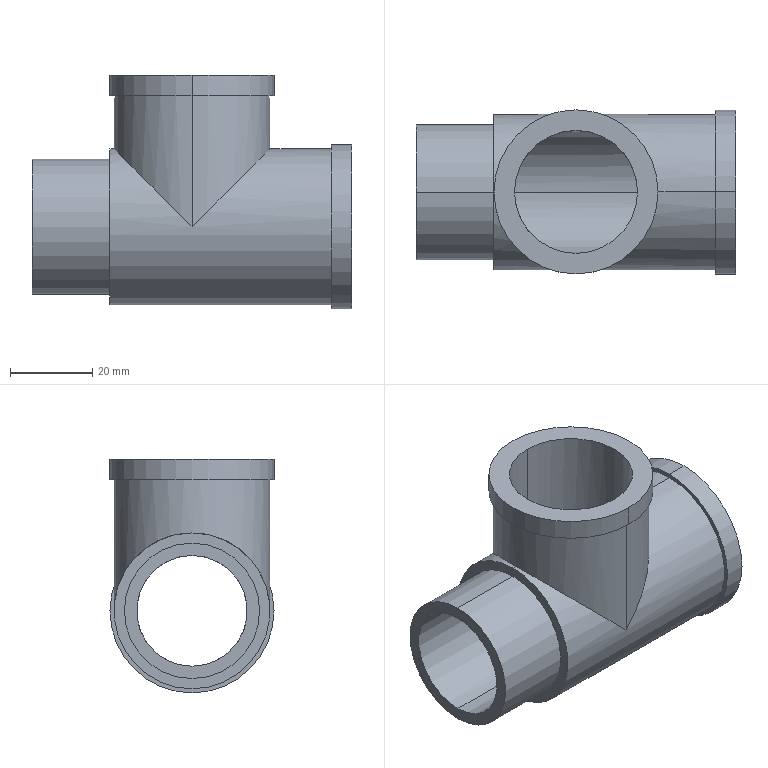Part | SolidWorks | features ICE 2, Revolution 2, Chamfer 1 | 1 solid | 26 faces | box 78 x 40 x 57 mm | volume 38567 mm3 | cylinder 18 | plane 8 | commonest cylinder face diameters 38 x6 30 x4 40 x4 27 x2 33 x2
STEP:
#1=CARTESIAN_POINT('',(78.,0.,-15.));
#2=VERTEX_POINT('',#1);
#3=CARTESIAN_POINT('',(78.,0.,15.));
#4=VERTEX_POINT('',#3);
#5=CARTESIAN_POINT('',(78.,0.,0.));
#6=DIRECTION('',(-1.,0.,0.));
#7=DIRECTION('',(0.,0.,1.));
#8=AXIS2_PLACEMENT_3D('',#5,#6,#7);
#9=CIRCLE('',#8,15.);
#10=EDGE_CURVE('',#2,#4,#9,.T.);
#11=ORIENTED_EDGE('',*,*,#10,.F.);
#12=CARTESIAN_POINT('',(20.,0.,-15.));
#13=VERTEX_POINT('',#12);
#14=CARTESIAN_POINT('',(0.,0.,-15.));
#15=DIRECTION('',(-1.,0.,0.));
#16=VECTOR('',#15,1000.);
#17=LINE('',#14,#16);
#18=EDGE_CURVE('',#2,#13,#17,.T.);
#19=ORIENTED_EDGE('',*,*,#18,.T.);
#20=CARTESIAN_POINT('',(21.,-6.083,-13.711));
#21=VERTEX_POINT('',#20);
#22=CARTESIAN_POINT('',(21.,-6.083,-13.711));
#23=CARTESIAN_POINT('',(20.843,-5.618,-13.918));
#24=CARTESIAN_POINT('',(20.701,-5.138,-14.102));
#25=CARTESIAN_POINT('',(20.455,-4.163,-14.42));
#26=CARTESIAN_POINT('',(20.35,-3.665,-14.555));
#27=CARTESIAN_POINT('',(20.178,-2.646,-14.774));
#28=CARTESIAN_POINT('',(20.112,-2.123,-14.858));
#29=CARTESIAN_POINT('',(20.023,-1.066,-14.972));
#30=CARTESIAN_POINT('',(20.,-0.5331,-15.));
#31=CARTESIAN_POINT('',(20.,0.,-15.));
#32=B_SPLINE_CURVE_WITH_KNOTS('',3,(#22,#23,#24,#25,#26,#27,#28,#29,#30,#31),.UNSPECIFIED.,.F.,.F.,(4,2,2,2,4),(0.09269,0.09426,0.09584,0.09741,0.09898),.UNSPECIFIED.);
#33=EDGE_CURVE('',#21,#13,#32,.T.);
#34=ORIENTED_EDGE('',*,*,#33,.F.);
#35=CARTESIAN_POINT('',(21.,-6.083,13.711));
#36=VERTEX_POINT('',#35);
#37=CARTESIAN_POINT('',(21.,0.,0.));
#38=DIRECTION('',(-1.,0.,0.));
#39=DIRECTION('',(0.,0.,1.));
#40=AXIS2_PLACEMENT_3D('',#37,#38,#39);
#41=CIRCLE('',#40,15.);
#42=EDGE_CURVE('',#21,#36,#41,.T.);
#43=ORIENTED_EDGE('',*,*,#42,.T.);
#44=CARTESIAN_POINT('',(20.,0.,15.));
#45=VERTEX_POINT('',#44);
#46=CARTESIAN_POINT('',(20.,0.,15.));
#47=CARTESIAN_POINT('',(20.,-0.5267,15.));
#48=CARTESIAN_POINT('',(20.022,-1.054,14.972));
#49=CARTESIAN_POINT('',(20.088,-1.844,14.889));
#50=CARTESIAN_POINT('',(20.116,-2.109,14.853));
#51=CARTESIAN_POINT('',(20.181,-2.632,14.77));
#52=CARTESIAN_POINT('',(20.219,-2.89,14.721));
#53=CARTESIAN_POINT('',(20.348,-3.657,14.557));
#54=CARTESIAN_POINT('',(20.453,-4.157,14.422));
#55=CARTESIAN_POINT('',(20.7,-5.136,14.103));
#56=CARTESIAN_POINT('',(20.843,-5.617,13.918));
#57=CARTESIAN_POINT('',(21.,-6.083,13.711));
#58=B_SPLINE_CURVE_WITH_KNOTS('',3,(#46,#47,#48,#49,#50,#51,#52,#53,#54,#55,#56,#57),.UNSPECIFIED.,.F.,.F.,(4,2,2,2,2,4),(0.04955,0.05113,0.05192,0.05271,0.05429,0.05587),.UNSPECIFIED.);
#59=EDGE_CURVE('',#45,#36,#58,.T.);
#60=ORIENTED_EDGE('',*,*,#59,.F.);
#61=CARTESIAN_POINT('',(24.,0.,15.));
#62=VERTEX_POINT('',#61);
#63=CARTESIAN_POINT('',(0.,0.,15.));
#64=DIRECTION('',(-1.,0.,0.));
#65=VECTOR('',#64,1000.);
#66=LINE('',#63,#65);
#67=EDGE_CURVE('',#62,#45,#66,.T.);
#68=ORIENTED_EDGE('',*,*,#67,.F.);
#69=CARTESIAN_POINT('',(39.,-15.,0.));
#70=VERTEX_POINT('',#69);
#71=CARTESIAN_POINT('',(39.,-15.,0.));
#72=CARTESIAN_POINT('',(30.213,-15.,8.787));
#73=CARTESIAN_POINT('',(24.,-8.787,15.));
#74=CARTESIAN_POINT('',(24.,0.,15.));
#75=(BOUNDED_CURVE()B_SPLINE_CURVE(3,(#71,#72,#73,#74),.UNSPECIFIED.,.F.,.F.)B_SPLINE_CURVE_WITH_KNOTS((4,4),(4.712,6.283),.UNSPECIFIED.)CURVE()GEOMETRIC_REPRESENTATION_ITEM()RATIONAL_B_SPLINE_CURVE((1.,0.8047,0.8047,1.))REPRESENTATION_ITEM(''));
#76=EDGE_CURVE('',#70,#62,#75,.T.);
#77=ORIENTED_EDGE('',*,*,#76,.F.);
#78=CARTESIAN_POINT('',(54.,0.,15.));
#79=VERTEX_POINT('',#78);
#80=CARTESIAN_POINT('',(54.,0.,15.));
#81=CARTESIAN_POINT('',(54.,-8.787,15.));
#82=CARTESIAN_POINT('',(47.787,-15.,8.787));
#83=CARTESIAN_POINT('',(39.,-15.,0.));
#84=(BOUNDED_CURVE()B_SPLINE_CURVE(3,(#80,#81,#82,#83),.UNSPECIFIED.,.F.,.F.)B_SPLINE_CURVE_WITH_KNOTS((4,4),(0.,1.571),.UNSPECIFIED.)CURVE()GEOMETRIC_REPRESENTATION_ITEM()RATIONAL_B_SPLINE_CURVE((1.,0.8047,0.8047,1.))REPRESENTATION_ITEM(''));
#85=EDGE_CURVE('',#79,#70,#84,.T.);
#86=ORIENTED_EDGE('',*,*,#85,.F.);
#87=CARTESIAN_POINT('',(0.,0.,15.));
#88=DIRECTION('',(-1.,0.,0.));
#89=VECTOR('',#88,1000.);
#90=LINE('',#87,#89);
#91=EDGE_CURVE('',#4,#79,#90,.T.);
#92=ORIENTED_EDGE('',*,*,#91,.F.);
#93=EDGE_LOOP('',(#11,#19,#34,#43,#60,#68,#77,#86,#92));
#94=FACE_OUTER_BOUND('',#93,.T.);
#95=CARTESIAN_POINT('',(0.,0.,0.));
#96=DIRECTION('',(-1.,0.,0.));
#97=DIRECTION('',(0.,0.,1.));
#98=AXIS2_PLACEMENT_3D('',#95,#96,#97);
#99=CYLINDRICAL_SURFACE('',#98,15.);
#100=ADVANCED_FACE('',(#94),#99,.F.);
#101=CARTESIAN_POINT('',(39.,-15.,37.));
#102=VERTEX_POINT('',#101);
#103=CARTESIAN_POINT('',(39.,15.,37.));
#104=VERTEX_POINT('',#103);
#105=CARTESIAN_POINT('',(39.,0.,37.));
#106=DIRECTION('',(0.,0.,-1.));
#107=DIRECTION('',(0.,1.,0.));
#108=AXIS2_PLACEMENT_3D('',#105,#106,#107);
#109=CIRCLE('',#108,15.);
#110=EDGE_CURVE('',#102,#104,#109,.T.);
#111=ORIENTED_EDGE('',*,*,#110,.F.);
#112=CARTESIAN_POINT('',(39.,-15.,0.));
#113=DIRECTION('',(0.,0.,-1.));
#114=VECTOR('',#113,1000.);
#115=LINE('',#112,#114);
#116=EDGE_CURVE('',#102,#70,#115,.T.);
#117=ORIENTED_EDGE('',*,*,#116,.T.);
#118=ORIENTED_EDGE('',*,*,#76,.T.);
#119=CARTESIAN_POINT('',(39.,15.,0.));
#120=VERTEX_POINT('',#119);
#121=CARTESIAN_POINT('',(24.,0.,15.));
#122=CARTESIAN_POINT('',(24.,8.787,15.));
#123=CARTESIAN_POINT('',(30.213,15.,8.787));
#124=CARTESIAN_POINT('',(39.,15.,0.));
#125=(BOUNDED_CURVE()B_SPLINE_CURVE(3,(#121,#122,#123,#124),.UNSPECIFIED.,.F.,.F.)B_SPLINE_CURVE_WITH_KNOTS((4,4),(0.,1.571),.UNSPECIFIED.)CURVE()GEOMETRIC_REPRESENTATION_ITEM()RATIONAL_B_SPLINE_CURVE((1.,0.8047,0.8047,1.))REPRESENTATION_ITEM(''));
#126=EDGE_CURVE('',#62,#120,#125,.T.);
#127=ORIENTED_EDGE('',*,*,#126,.T.);
#128=CARTESIAN_POINT('',(39.,15.,0.));
#129=DIRECTION('',(0.,0.,-1.));
#130=VECTOR('',#129,1000.);
#131=LINE('',#128,#130);
#132=EDGE_CURVE('',#104,#120,#131,.T.);
#133=ORIENTED_EDGE('',*,*,#132,.F.);
#134=EDGE_LOOP('',(#111,#117,#118,#127,#133));
#135=FACE_OUTER_BOUND('',#134,.T.);
#136=CARTESIAN_POINT('',(39.,0.,0.));
#137=DIRECTION('',(0.,0.,-1.));
#138=DIRECTION('',(0.,1.,0.));
#139=AXIS2_PLACEMENT_3D('',#136,#137,#138);
#140=CYLINDRICAL_SURFACE('',#139,15.);
#141=ADVANCED_FACE('',(#135),#140,.F.);
#142=CARTESIAN_POINT('',(39.,19.,32.));
#143=VERTEX_POINT('',#142);
#144=CARTESIAN_POINT('',(39.,-19.,32.));
#145=VERTEX_POINT('',#144);
#146=CARTESIAN_POINT('',(39.,0.,32.));
#147=DIRECTION('',(0.,0.,-1.));
#148=DIRECTION('',(0.,1.,0.));
#149=AXIS2_PLACEMENT_3D('',#146,#147,#148);
#150=CIRCLE('',#149,19.);
#151=EDGE_CURVE('',#143,#145,#150,.T.);
#152=ORIENTED_EDGE('',*,*,#151,.T.);
#153=CARTESIAN_POINT('',(39.,-19.,0.));
#154=VERTEX_POINT('',#153);
#155=CARTESIAN_POINT('',(39.,-19.,0.));
#156=DIRECTION('',(0.,0.,-1.));
#157=VECTOR('',#156,1000.);
#158=LINE('',#155,#157);
#159=EDGE_CURVE('',#145,#154,#158,.T.);
#160=ORIENTED_EDGE('',*,*,#159,.T.);
#161=CARTESIAN_POINT('',(58.,0.,19.));
#162=VERTEX_POINT('',#161);
#163=CARTESIAN_POINT('',(39.,-19.,0.));
#164=CARTESIAN_POINT('',(50.13,-19.,11.13));
#165=CARTESIAN_POINT('',(58.,-11.13,19.));
#166=CARTESIAN_POINT('',(58.,0.,19.));
#167=(BOUNDED_CURVE()B_SPLINE_CURVE(3,(#163,#164,#165,#166),.UNSPECIFIED.,.F.,.T.)B_SPLINE_CURVE_WITH_KNOTS((4,4),(1.571,3.142),.UNSPECIFIED.)CURVE()GEOMETRIC_REPRESENTATION_ITEM()RATIONAL_B_SPLINE_CURVE((1.,0.8047,0.8047,1.))REPRESENTATION_ITEM(''));
#168=EDGE_CURVE('',#154,#162,#167,.T.);
#169=ORIENTED_EDGE('',*,*,#168,.T.);
#170=CARTESIAN_POINT('',(39.,19.,0.));
#171=VERTEX_POINT('',#170);
#172=CARTESIAN_POINT('',(58.,0.,19.));
#173=CARTESIAN_POINT('',(58.,11.13,19.));
#174=CARTESIAN_POINT('',(50.13,19.,11.13));
#175=CARTESIAN_POINT('',(39.,19.,0.));
#176=(BOUNDED_CURVE()B_SPLINE_CURVE(3,(#172,#173,#174,#175),.UNSPECIFIED.,.F.,.F.)B_SPLINE_CURVE_WITH_KNOTS((4,4),(3.142,4.712),.UNSPECIFIED.)CURVE()GEOMETRIC_REPRESENTATION_ITEM()RATIONAL_B_SPLINE_CURVE((1.,0.8047,0.8047,1.))REPRESENTATION_ITEM(''));
#177=EDGE_CURVE('',#162,#171,#176,.T.);
#178=ORIENTED_EDGE('',*,*,#177,.T.);
#179=CARTESIAN_POINT('',(39.,19.,0.));
#180=DIRECTION('',(0.,0.,-1.));
#181=VECTOR('',#180,1000.);
#182=LINE('',#179,#181);
#183=EDGE_CURVE('',#143,#171,#182,.T.);
#184=ORIENTED_EDGE('',*,*,#183,.F.);
#185=EDGE_LOOP('',(#152,#160,#169,#178,#184));
#186=FACE_OUTER_BOUND('',#185,.T.);
#187=CARTESIAN_POINT('',(39.,0.,0.));
#188=DIRECTION('',(0.,0.,-1.));
#189=DIRECTION('',(0.,1.,0.));
#190=AXIS2_PLACEMENT_3D('',#187,#188,#189);
#191=CYLINDRICAL_SURFACE('',#190,19.);
#192=ADVANCED_FACE('',(#186),#191,.T.);
#193=CARTESIAN_POINT('',(39.,20.,37.));
#194=VERTEX_POINT('',#193);
#195=CARTESIAN_POINT('',(39.,-20.,37.));
#196=VERTEX_POINT('',#195);
#197=CARTESIAN_POINT('',(39.,0.,37.));
#198=DIRECTION('',(0.,0.,-1.));
#199=DIRECTION('',(0.,1.,0.));
#200=AXIS2_PLACEMENT_3D('',#197,#198,#199);
#201=CIRCLE('',#200,20.);
#202=EDGE_CURVE('',#194,#196,#201,.T.);
#203=ORIENTED_EDGE('',*,*,#202,.T.);
#204=CARTESIAN_POINT('',(39.,-20.,32.));
#205=VERTEX_POINT('',#204);
#206=CARTESIAN_POINT('',(39.,-20.,0.));
#207=DIRECTION('',(0.,0.,-1.));
#208=VECTOR('',#207,1000.);
#209=LINE('',#206,#208);
#210=EDGE_CURVE('',#196,#205,#209,.T.);
#211=ORIENTED_EDGE('',*,*,#210,.T.);
#212=CARTESIAN_POINT('',(39.,20.,32.));
#213=VERTEX_POINT('',#212);
#214=CARTESIAN_POINT('',(39.,0.,32.));
#215=DIRECTION('',(0.,0.,-1.));
#216=DIRECTION('',(0.,1.,0.));
#217=AXIS2_PLACEMENT_3D('',#214,#215,#216);
#218=CIRCLE('',#217,20.);
#219=EDGE_CURVE('',#213,#205,#218,.T.);
#220=ORIENTED_EDGE('',*,*,#219,.F.);
#221=CARTESIAN_POINT('',(39.,20.,0.));
#222=DIRECTION('',(0.,0.,-1.));
#223=VECTOR('',#222,1000.);
#224=LINE('',#221,#223);
#225=EDGE_CURVE('',#194,#213,#224,.T.);
#226=ORIENTED_EDGE('',*,*,#225,.F.);
#227=EDGE_LOOP('',(#203,#211,#220,#226));
#228=FACE_OUTER_BOUND('',#227,.T.);
#229=CARTESIAN_POINT('',(39.,0.,0.));
#230=DIRECTION('',(0.,0.,-1.));
#231=DIRECTION('',(0.,1.,0.));
#232=AXIS2_PLACEMENT_3D('',#229,#230,#231);
#233=CYLINDRICAL_SURFACE('',#232,20.);
#234=ADVANCED_FACE('',(#228),#233,.T.);
#235=CARTESIAN_POINT('',(78.,0.,20.));
#236=VERTEX_POINT('',#235);
#237=CARTESIAN_POINT('',(78.,0.,-20.));
#238=VERTEX_POINT('',#237);
#239=CARTESIAN_POINT('',(78.,0.,0.));
#240=DIRECTION('',(-1.,0.,0.));
#241=DIRECTION('',(0.,0.,1.));
#242=AXIS2_PLACEMENT_3D('',#239,#240,#241);
#243=CIRCLE('',#242,20.);
#244=EDGE_CURVE('',#236,#238,#243,.T.);
#245=ORIENTED_EDGE('',*,*,#244,.T.);
#246=CARTESIAN_POINT('',(73.,0.,-20.));
#247=VERTEX_POINT('',#246);
#248=CARTESIAN_POINT('',(0.,0.,-20.));
#249=DIRECTION('',(-1.,0.,0.));
#250=VECTOR('',#249,1000.);
#251=LINE('',#248,#250);
#252=EDGE_CURVE('',#238,#247,#251,.T.);
#253=ORIENTED_EDGE('',*,*,#252,.T.);
#254=CARTESIAN_POINT('',(73.,0.,20.));
#255=VERTEX_POINT('',#254);
#256=CARTESIAN_POINT('',(73.,0.,0.));
#257=DIRECTION('',(-1.,0.,0.));
#258=DIRECTION('',(0.,0.,1.));
#259=AXIS2_PLACEMENT_3D('',#256,#257,#258);
#260=CIRCLE('',#259,20.);
#261=EDGE_CURVE('',#255,#247,#260,.T.);
#262=ORIENTED_EDGE('',*,*,#261,.F.);
#263=CARTESIAN_POINT('',(0.,0.,20.));
#264=DIRECTION('',(-1.,0.,0.));
#265=VECTOR('',#264,1000.);
#266=LINE('',#263,#265);
#267=EDGE_CURVE('',#236,#255,#266,.T.);
#268=ORIENTED_EDGE('',*,*,#267,.F.);
#269=EDGE_LOOP('',(#245,#253,#262,#268));
#270=FACE_OUTER_BOUND('',#269,.T.);
#271=CARTESIAN_POINT('',(0.,0.,0.));
#272=DIRECTION('',(-1.,0.,0.));
#273=DIRECTION('',(0.,0.,1.));
#274=AXIS2_PLACEMENT_3D('',#271,#272,#273);
#275=CYLINDRICAL_SURFACE('',#274,20.);
#276=ADVANCED_FACE('',(#270),#275,.T.);
#277=CARTESIAN_POINT('',(19.,0.,16.5));
#278=VERTEX_POINT('',#277);
#279=CARTESIAN_POINT('',(19.,0.,-16.5));
#280=VERTEX_POINT('',#279);
#281=CARTESIAN_POINT('',(19.,0.,0.));
#282=DIRECTION('',(-1.,0.,0.));
#283=DIRECTION('',(0.,0.,1.));
#284=AXIS2_PLACEMENT_3D('',#281,#282,#283);
#285=CIRCLE('',#284,16.5);
#286=EDGE_CURVE('',#278,#280,#285,.T.);
#287=ORIENTED_EDGE('',*,*,#286,.T.);
#288=CARTESIAN_POINT('',(0.,0.,-16.5));
#289=VERTEX_POINT('',#288);
#290=CARTESIAN_POINT('',(0.,0.,-16.5));
#291=DIRECTION('',(-1.,0.,0.));
#292=VECTOR('',#291,1000.);
#293=LINE('',#290,#292);
#294=EDGE_CURVE('',#280,#289,#293,.T.);
#295=ORIENTED_EDGE('',*,*,#294,.T.);
#296=CARTESIAN_POINT('',(0.,0.,16.5));
#297=VERTEX_POINT('',#296);
#298=CARTESIAN_POINT('',(0.,0.,0.));
#299=DIRECTION('',(-1.,0.,0.));
#300=DIRECTION('',(0.,0.,1.));
#301=AXIS2_PLACEMENT_3D('',#298,#299,#300);
#302=CIRCLE('',#301,16.5);
#303=EDGE_CURVE('',#297,#289,#302,.T.);
#304=ORIENTED_EDGE('',*,*,#303,.F.);
#305=CARTESIAN_POINT('',(0.,0.,16.5));
#306=DIRECTION('',(-1.,0.,0.));
#307=VECTOR('',#306,1000.);
#308=LINE('',#305,#307);
#309=EDGE_CURVE('',#278,#297,#308,.T.);
#310=ORIENTED_EDGE('',*,*,#309,.F.);
#311=EDGE_LOOP('',(#287,#295,#304,#310));
#312=FACE_OUTER_BOUND('',#311,.T.);
#313=CARTESIAN_POINT('',(0.,0.,0.));
#314=DIRECTION('',(-1.,0.,0.));
#315=DIRECTION('',(0.,0.,1.));
#316=AXIS2_PLACEMENT_3D('',#313,#314,#315);
#317=CYLINDRICAL_SURFACE('',#316,16.5);
#318=ADVANCED_FACE('',(#312),#317,.T.);
#319=CARTESIAN_POINT('',(73.,0.,19.));
#320=VERTEX_POINT('',#319);
#321=CARTESIAN_POINT('',(73.,0.,-19.));
#322=VERTEX_POINT('',#321);
#323=CARTESIAN_POINT('',(73.,0.,0.));
#324=DIRECTION('',(-1.,0.,0.));
#325=DIRECTION('',(0.,0.,1.));
#326=AXIS2_PLACEMENT_3D('',#323,#324,#325);
#327=CIRCLE('',#326,19.);
#328=EDGE_CURVE('',#320,#322,#327,.T.);
#329=ORIENTED_EDGE('',*,*,#328,.T.);
#330=CARTESIAN_POINT('',(19.,0.,-19.));
#331=VERTEX_POINT('',#330);
#332=CARTESIAN_POINT('',(0.,0.,-19.));
#333=DIRECTION('',(-1.,0.,0.));
#334=VECTOR('',#333,1000.);
#335=LINE('',#332,#334);
#336=EDGE_CURVE('',#322,#331,#335,.T.);
#337=ORIENTED_EDGE('',*,*,#336,.T.);
#338=CARTESIAN_POINT('',(19.,0.,19.));
#339=VERTEX_POINT('',#338);
#340=CARTESIAN_POINT('',(19.,0.,0.));
#341=DIRECTION('',(-1.,0.,0.));
#342=DIRECTION('',(0.,0.,1.));
#343=AXIS2_PLACEMENT_3D('',#340,#341,#342);
#344=CIRCLE('',#343,19.);
#345=EDGE_CURVE('',#339,#331,#344,.T.);
#346=ORIENTED_EDGE('',*,*,#345,.F.);
#347=CARTESIAN_POINT('',(20.,0.,19.));
#348=VERTEX_POINT('',#347);
#349=CARTESIAN_POINT('',(0.,0.,19.));
#350=DIRECTION('',(-1.,0.,0.));
#351=VECTOR('',#350,1000.);
#352=LINE('',#349,#351);
#353=EDGE_CURVE('',#348,#339,#352,.T.);
#354=ORIENTED_EDGE('',*,*,#353,.F.);
#355=CARTESIAN_POINT('',(39.,19.,0.));
#356=CARTESIAN_POINT('',(27.87,19.,11.13));
#357=CARTESIAN_POINT('',(20.,11.13,19.));
#358=CARTESIAN_POINT('',(20.,0.,19.));
#359=(BOUNDED_CURVE()B_SPLINE_CURVE(3,(#355,#356,#357,#358),.UNSPECIFIED.,.F.,.F.)B_SPLINE_CURVE_WITH_KNOTS((4,4),(4.712,6.283),.UNSPECIFIED.)CURVE()GEOMETRIC_REPRESENTATION_ITEM()RATIONAL_B_SPLINE_CURVE((1.,0.8047,0.8047,1.))REPRESENTATION_ITEM(''));
#360=EDGE_CURVE('',#171,#348,#359,.T.);
#361=ORIENTED_EDGE('',*,*,#360,.F.);
#362=ORIENTED_EDGE('',*,*,#177,.F.);
#363=CARTESIAN_POINT('',(0.,0.,19.));
#364=DIRECTION('',(-1.,0.,0.));
#365=VECTOR('',#364,1000.);
#366=LINE('',#363,#365);
#367=EDGE_CURVE('',#320,#162,#366,.T.);
#368=ORIENTED_EDGE('',*,*,#367,.F.);
#369=EDGE_LOOP('',(#329,#337,#346,#354,#361,#362,#368));
#370=FACE_OUTER_BOUND('',#369,.T.);
#371=CARTESIAN_POINT('',(0.,0.,0.));
#372=DIRECTION('',(-1.,0.,0.));
#373=DIRECTION('',(0.,0.,1.));
#374=AXIS2_PLACEMENT_3D('',#371,#372,#373);
#375=CYLINDRICAL_SURFACE('',#374,19.);
#376=ADVANCED_FACE('',(#370),#375,.T.);
#377=CARTESIAN_POINT('',(20.,0.,-13.5));
#378=VERTEX_POINT('',#377);
#379=CARTESIAN_POINT('',(21.,-6.083,-12.052));
#380=VERTEX_POINT('',#379);
#381=CARTESIAN_POINT('',(20.,0.,-13.5));
#382=CARTESIAN_POINT('',(20.,-0.5304,-13.5));
#383=CARTESIAN_POINT('',(20.022,-1.064,-13.469));
#384=CARTESIAN_POINT('',(20.112,-2.128,-13.342));
#385=CARTESIAN_POINT('',(20.178,-2.649,-13.248));
#386=CARTESIAN_POINT('',(20.35,-3.668,-13.003));
#387=CARTESIAN_POINT('',(20.456,-4.168,-12.851));
#388=CARTESIAN_POINT('',(20.703,-5.146,-12.492));
#389=CARTESIAN_POINT('',(20.845,-5.623,-12.284));
#390=CARTESIAN_POINT('',(21.,-6.083,-12.052));
#391=B_SPLINE_CURVE_WITH_KNOTS('',3,(#381,#382,#383,#384,#385,#386,#387,#388,#389,#390),.UNSPECIFIED.,.F.,.F.,(4,2,2,2,4),(0.006389,0.007982,0.009575,0.01117,0.01276),.UNSPECIFIED.);
#392=EDGE_CURVE('',#378,#380,#391,.T.);
#393=ORIENTED_EDGE('',*,*,#392,.F.);
#394=CARTESIAN_POINT('',(0.,0.,-13.5));
#395=VERTEX_POINT('',#394);
#396=CARTESIAN_POINT('',(0.,0.,-13.5));
#397=DIRECTION('',(-1.,0.,0.));
#398=VECTOR('',#397,1000.);
#399=LINE('',#396,#398);
#400=EDGE_CURVE('',#378,#395,#399,.T.);
#401=ORIENTED_EDGE('',*,*,#400,.T.);
#402=CARTESIAN_POINT('',(0.,0.,13.5));
#403=VERTEX_POINT('',#402);
#404=CARTESIAN_POINT('',(0.,0.,0.));
#405=DIRECTION('',(-1.,0.,0.));
#406=DIRECTION('',(0.,0.,1.));
#407=AXIS2_PLACEMENT_3D('',#404,#405,#406);
#408=CIRCLE('',#407,13.5);
#409=EDGE_CURVE('',#395,#403,#408,.T.);
#410=ORIENTED_EDGE('',*,*,#409,.T.);
#411=CARTESIAN_POINT('',(20.,0.,13.5));
#412=VERTEX_POINT('',#411);
#413=CARTESIAN_POINT('',(0.,0.,13.5));
#414=DIRECTION('',(-1.,0.,0.));
#415=VECTOR('',#414,1000.);
#416=LINE('',#413,#415);
#417=EDGE_CURVE('',#412,#403,#416,.T.);
#418=ORIENTED_EDGE('',*,*,#417,.F.);
#419=CARTESIAN_POINT('',(21.,-6.083,12.052));
#420=VERTEX_POINT('',#419);
#421=CARTESIAN_POINT('',(21.,-6.083,12.052));
#422=CARTESIAN_POINT('',(20.847,-5.631,12.28));
#423=CARTESIAN_POINT('',(20.708,-5.162,12.485));
#424=CARTESIAN_POINT('',(20.46,-4.187,12.845));
#425=CARTESIAN_POINT('',(20.352,-3.677,13.));
#426=CARTESIAN_POINT('',(20.178,-2.649,13.248));
#427=CARTESIAN_POINT('',(20.112,-2.129,13.342));
#428=CARTESIAN_POINT('',(20.023,-1.075,13.468));
#429=CARTESIAN_POINT('',(20.,-0.5395,13.5));
#430=CARTESIAN_POINT('',(20.,0.,13.5));
#431=B_SPLINE_CURVE_WITH_KNOTS('',3,(#421,#422,#423,#424,#425,#426,#427,#428,#429,#430),.UNSPECIFIED.,.F.,.F.,(4,2,2,2,4),(0.08145,0.08304,0.08463,0.08622,0.08782),.UNSPECIFIED.);
#432=EDGE_CURVE('',#420,#412,#431,.T.);
#433=ORIENTED_EDGE('',*,*,#432,.F.);
#434=CARTESIAN_POINT('',(21.,0.,0.));
#435=DIRECTION('',(-1.,0.,0.));
#436=DIRECTION('',(0.,0.,1.));
#437=AXIS2_PLACEMENT_3D('',#434,#435,#436);
#438=CIRCLE('',#437,13.5);
#439=EDGE_CURVE('',#380,#420,#438,.T.);
#440=ORIENTED_EDGE('',*,*,#439,.F.);
#441=EDGE_LOOP('',(#393,#401,#410,#418,#433,#440));
#442=FACE_OUTER_BOUND('',#441,.T.);
#443=CARTESIAN_POINT('',(0.,0.,0.));
#444=DIRECTION('',(-1.,0.,0.));
#445=DIRECTION('',(0.,0.,1.));
#446=AXIS2_PLACEMENT_3D('',#443,#444,#445);
#447=CYLINDRICAL_SURFACE('',#446,13.5);
#448=ADVANCED_FACE('',(#442),#447,.F.);
#449=ORIENTED_EDGE('',*,*,#400,.F.);
#450=CARTESIAN_POINT('',(21.,6.083,-12.052));
#451=VERTEX_POINT('',#450);
#452=CARTESIAN_POINT('',(21.,6.083,-12.052));
#453=CARTESIAN_POINT('',(20.689,5.161,-12.517));
#454=CARTESIAN_POINT('',(20.438,4.19,-12.877));
#455=CARTESIAN_POINT('',(20.178,2.649,-13.248));
#456=CARTESIAN_POINT('',(20.111,2.119,-13.343));
#457=CARTESIAN_POINT('',(20.022,1.062,-13.469));
#458=CARTESIAN_POINT('',(20.,0.5319,-13.5));
#459=CARTESIAN_POINT('',(20.,0.,-13.5));
#460=B_SPLINE_CURVE_WITH_KNOTS('',3,(#452,#453,#454,#455,#456,#457,#458,#459),.UNSPECIFIED.,.F.,.F.,(4,2,2,4),(0.,0.003195,0.004792,0.006389),.UNSPECIFIED.);
#461=EDGE_CURVE('',#451,#378,#460,.T.);
#462=ORIENTED_EDGE('',*,*,#461,.F.);
#463=CARTESIAN_POINT('',(21.,6.083,12.052));
#464=VERTEX_POINT('',#463);
#465=CARTESIAN_POINT('',(21.,0.,0.));
#466=DIRECTION('',(-1.,0.,0.));
#467=DIRECTION('',(0.,0.,1.));
#468=AXIS2_PLACEMENT_3D('',#465,#466,#467);
#469=CIRCLE('',#468,13.5);
#470=EDGE_CURVE('',#464,#451,#469,.T.);
#471=ORIENTED_EDGE('',*,*,#470,.F.);
#472=CARTESIAN_POINT('',(20.,0.,13.5));
#473=CARTESIAN_POINT('',(20.,1.08,13.5));
#474=CARTESIAN_POINT('',(20.091,2.132,13.372));
#475=CARTESIAN_POINT('',(20.351,3.67,13.002));
#476=CARTESIAN_POINT('',(20.458,4.179,12.848));
#477=CARTESIAN_POINT('',(20.706,5.156,12.488));
#478=CARTESIAN_POINT('',(20.846,5.627,12.282));
#479=CARTESIAN_POINT('',(21.,6.083,12.052));
#480=B_SPLINE_CURVE_WITH_KNOTS('',3,(#472,#473,#474,#475,#476,#477,#478,#479),.UNSPECIFIED.,.F.,.F.,(4,2,2,4),(0.,0.003188,0.004782,0.006376),.UNSPECIFIED.);
#481=EDGE_CURVE('',#412,#464,#480,.T.);
#482=ORIENTED_EDGE('',*,*,#481,.F.);
#483=ORIENTED_EDGE('',*,*,#417,.T.);
#484=CARTESIAN_POINT('',(0.,0.,0.));
#485=DIRECTION('',(-1.,0.,0.));
#486=DIRECTION('',(0.,0.,1.));
#487=AXIS2_PLACEMENT_3D('',#484,#485,#486);
#488=CIRCLE('',#487,13.5);
#489=EDGE_CURVE('',#403,#395,#488,.T.);
#490=ORIENTED_EDGE('',*,*,#489,.T.);
#491=EDGE_LOOP('',(#449,#462,#471,#482,#483,#490));
#492=FACE_OUTER_BOUND('',#491,.T.);
#493=CARTESIAN_POINT('',(0.,0.,0.));
#494=DIRECTION('',(-1.,0.,0.));
#495=DIRECTION('',(0.,0.,1.));
#496=AXIS2_PLACEMENT_3D('',#493,#494,#495);
#497=CYLINDRICAL_SURFACE('',#496,13.5);
#498=ADVANCED_FACE('',(#492),#497,.F.);
#499=CARTESIAN_POINT('',(21.,6.083,-13.711));
#500=VERTEX_POINT('',#499);
#501=CARTESIAN_POINT('',(21.,6.083,0.));
#502=DIRECTION('',(0.,0.,1.));
#503=VECTOR('',#502,1000.);
#504=LINE('',#501,#503);
#505=EDGE_CURVE('',#500,#451,#504,.T.);
#506=ORIENTED_EDGE('',*,*,#505,.F.);
#507=CARTESIAN_POINT('',(21.,6.083,13.711));
#508=VERTEX_POINT('',#507);
#509=CARTESIAN_POINT('',(21.,0.,0.));
#510=DIRECTION('',(-1.,0.,0.));
#511=DIRECTION('',(0.,0.,1.));
#512=AXIS2_PLACEMENT_3D('',#509,#510,#511);
#513=CIRCLE('',#512,15.);
#514=EDGE_CURVE('',#508,#500,#513,.T.);
#515=ORIENTED_EDGE('',*,*,#514,.F.);
#516=CARTESIAN_POINT('',(21.,6.083,0.));
#517=DIRECTION('',(0.,0.,1.));
#518=VECTOR('',#517,1000.);
#519=LINE('',#516,#518);
#520=EDGE_CURVE('',#464,#508,#519,.T.);
#521=ORIENTED_EDGE('',*,*,#520,.F.);
#522=ORIENTED_EDGE('',*,*,#470,.T.);
#523=EDGE_LOOP('',(#506,#515,#521,#522));
#524=FACE_OUTER_BOUND('',#523,.T.);
#525=CARTESIAN_POINT('',(21.,15.,0.));
#526=DIRECTION('',(-1.,0.,0.));
#527=DIRECTION('',(0.,0.,1.));
#528=AXIS2_PLACEMENT_3D('',#525,#526,#527);
#529=PLANE('',#528);
#530=ADVANCED_FACE('',(#524),#529,.F.);
#531=CARTESIAN_POINT('',(21.,-6.083,0.));
#532=DIRECTION('',(0.,0.,-1.));
#533=VECTOR('',#532,1000.);
#534=LINE('',#531,#533);
#535=EDGE_CURVE('',#380,#21,#534,.T.);
#536=ORIENTED_EDGE('',*,*,#535,.F.);
#537=ORIENTED_EDGE('',*,*,#439,.T.);
#538=CARTESIAN_POINT('',(21.,-6.083,0.));
#539=DIRECTION('',(0.,0.,-1.));
#540=VECTOR('',#539,1000.);
#541=LINE('',#538,#540);
#542=EDGE_CURVE('',#36,#420,#541,.T.);
#543=ORIENTED_EDGE('',*,*,#542,.F.);
#544=ORIENTED_EDGE('',*,*,#42,.F.);
#545=EDGE_LOOP('',(#536,#537,#543,#544));
#546=FACE_OUTER_BOUND('',#545,.T.);
#547=CARTESIAN_POINT('',(21.,15.,0.));
#548=DIRECTION('',(-1.,0.,0.));
#549=DIRECTION('',(0.,0.,1.));
#550=AXIS2_PLACEMENT_3D('',#547,#548,#549);
#551=PLANE('',#550);
#552=ADVANCED_FACE('',(#546),#551,.F.);
#553=ORIENTED_EDGE('',*,*,#336,.F.);
#554=CARTESIAN_POINT('',(73.,0.,0.));
#555=DIRECTION('',(-1.,0.,0.));
#556=DIRECTION('',(0.,0.,1.));
#557=AXIS2_PLACEMENT_3D('',#554,#555,#556);
#558=CIRCLE('',#557,19.);
#559=EDGE_CURVE('',#322,#320,#558,.T.);
#560=ORIENTED_EDGE('',*,*,#559,.T.);
#561=ORIENTED_EDGE('',*,*,#367,.T.);
#562=ORIENTED_EDGE('',*,*,#168,.F.);
#563=CARTESIAN_POINT('',(20.,0.,19.));
#564=CARTESIAN_POINT('',(20.,-11.13,19.));
#565=CARTESIAN_POINT('',(27.87,-19.,11.13));
#566=CARTESIAN_POINT('',(39.,-19.,0.));
#567=(BOUNDED_CURVE()B_SPLINE_CURVE(3,(#563,#564,#565,#566),.UNSPECIFIED.,.F.,.T.)B_SPLINE_CURVE_WITH_KNOTS((4,4),(0.,1.571),.UNSPECIFIED.)CURVE()GEOMETRIC_REPRESENTATION_ITEM()RATIONAL_B_SPLINE_CURVE((1.,0.8047,0.8047,1.))REPRESENTATION_ITEM(''));
#568=EDGE_CURVE('',#348,#154,#567,.T.);
#569=ORIENTED_EDGE('',*,*,#568,.F.);
#570=ORIENTED_EDGE('',*,*,#353,.T.);
#571=CARTESIAN_POINT('',(19.,0.,0.));
#572=DIRECTION('',(-1.,0.,0.));
#573=DIRECTION('',(0.,0.,1.));
#574=AXIS2_PLACEMENT_3D('',#571,#572,#573);
#575=CIRCLE('',#574,19.);
#576=EDGE_CURVE('',#331,#339,#575,.T.);
#577=ORIENTED_EDGE('',*,*,#576,.F.);
#578=EDGE_LOOP('',(#553,#560,#561,#562,#569,#570,#577));
#579=FACE_OUTER_BOUND('',#578,.T.);
#580=CARTESIAN_POINT('',(0.,0.,0.));
#581=DIRECTION('',(-1.,0.,0.));
#582=DIRECTION('',(0.,0.,1.));
#583=AXIS2_PLACEMENT_3D('',#580,#581,#582);
#584=CYLINDRICAL_SURFACE('',#583,19.);
#585=ADVANCED_FACE('',(#579),#584,.T.);
#586=ORIENTED_EDGE('',*,*,#294,.F.);
#587=CARTESIAN_POINT('',(19.,0.,0.));
#588=DIRECTION('',(-1.,0.,0.));
#589=DIRECTION('',(0.,0.,1.));
#590=AXIS2_PLACEMENT_3D('',#587,#588,#589);
#591=CIRCLE('',#590,16.5);
#592=EDGE_CURVE('',#280,#278,#591,.T.);
#593=ORIENTED_EDGE('',*,*,#592,.T.);
#594=ORIENTED_EDGE('',*,*,#309,.T.);
#595=CARTESIAN_POINT('',(0.,0.,0.));
#596=DIRECTION('',(-1.,0.,0.));
#597=DIRECTION('',(0.,0.,1.));
#598=AXIS2_PLACEMENT_3D('',#595,#596,#597);
#599=CIRCLE('',#598,16.5);
#600=EDGE_CURVE('',#289,#297,#599,.T.);
#601=ORIENTED_EDGE('',*,*,#600,.F.);
#602=EDGE_LOOP('',(#586,#593,#594,#601));
#603=FACE_OUTER_BOUND('',#602,.T.);
#604=CARTESIAN_POINT('',(0.,0.,0.));
#605=DIRECTION('',(-1.,0.,0.));
#606=DIRECTION('',(0.,0.,1.));
#607=AXIS2_PLACEMENT_3D('',#604,#605,#606);
#608=CYLINDRICAL_SURFACE('',#607,16.5);
#609=ADVANCED_FACE('',(#603),#608,.T.);
#610=ORIENTED_EDGE('',*,*,#489,.F.);
#611=ORIENTED_EDGE('',*,*,#409,.F.);
#612=EDGE_LOOP('',(#610,#611));
#613=FACE_BOUND('',#612,.T.);
#614=ORIENTED_EDGE('',*,*,#303,.T.);
#615=ORIENTED_EDGE('',*,*,#600,.T.);
#616=EDGE_LOOP('',(#614,#615));
#617=FACE_OUTER_BOUND('',#616,.T.);
#618=CARTESIAN_POINT('',(0.,16.5,0.));
#619=DIRECTION('',(1.,0.,0.));
#620=DIRECTION('',(0.,0.,-1.));
#621=AXIS2_PLACEMENT_3D('',#618,#619,#620);
#622=PLANE('',#621);
#623=ADVANCED_FACE('',(#613,#617),#622,.F.);
#624=ORIENTED_EDGE('',*,*,#244,.F.);
#625=CARTESIAN_POINT('',(78.,0.,0.));
#626=DIRECTION('',(-1.,0.,0.));
#627=DIRECTION('',(0.,0.,1.));
#628=AXIS2_PLACEMENT_3D('',#625,#626,#627);
#629=CIRCLE('',#628,20.);
#630=EDGE_CURVE('',#238,#236,#629,.T.);
#631=ORIENTED_EDGE('',*,*,#630,.F.);
#632=EDGE_LOOP('',(#624,#631));
#633=FACE_OUTER_BOUND('',#632,.T.);
#634=CARTESIAN_POINT('',(78.,0.,0.));
#635=DIRECTION('',(-1.,0.,0.));
#636=DIRECTION('',(0.,0.,1.));
#637=AXIS2_PLACEMENT_3D('',#634,#635,#636);
#638=CIRCLE('',#637,15.);
#639=EDGE_CURVE('',#4,#2,#638,.T.);
#640=ORIENTED_EDGE('',*,*,#639,.T.);
#641=ORIENTED_EDGE('',*,*,#10,.T.);
#642=EDGE_LOOP('',(#640,#641));
#643=FACE_BOUND('',#642,.T.);
#644=CARTESIAN_POINT('',(78.,20.,0.));
#645=DIRECTION('',(-1.,0.,0.));
#646=DIRECTION('',(0.,0.,1.));
#647=AXIS2_PLACEMENT_3D('',#644,#645,#646);
#648=PLANE('',#647);
#649=ADVANCED_FACE('',(#633,#643),#648,.F.);
#650=ORIENTED_EDGE('',*,*,#252,.F.);
#651=ORIENTED_EDGE('',*,*,#630,.T.);
#652=ORIENTED_EDGE('',*,*,#267,.T.);
#653=CARTESIAN_POINT('',(73.,0.,0.));
#654=DIRECTION('',(-1.,0.,0.));
#655=DIRECTION('',(0.,0.,1.));
#656=AXIS2_PLACEMENT_3D('',#653,#654,#655);
#657=CIRCLE('',#656,20.);
#658=EDGE_CURVE('',#247,#255,#657,.T.);
#659=ORIENTED_EDGE('',*,*,#658,.F.);
#660=EDGE_LOOP('',(#650,#651,#652,#659));
#661=FACE_OUTER_BOUND('',#660,.T.);
#662=CARTESIAN_POINT('',(0.,0.,0.));
#663=DIRECTION('',(-1.,0.,0.));
#664=DIRECTION('',(0.,0.,1.));
#665=AXIS2_PLACEMENT_3D('',#662,#663,#664);
#666=CYLINDRICAL_SURFACE('',#665,20.);
#667=ADVANCED_FACE('',(#661),#666,.T.);
#668=ORIENTED_EDGE('',*,*,#328,.F.);
#669=ORIENTED_EDGE('',*,*,#559,.F.);
#670=EDGE_LOOP('',(#668,#669));
#671=FACE_BOUND('',#670,.T.);
#672=ORIENTED_EDGE('',*,*,#261,.T.);
#673=ORIENTED_EDGE('',*,*,#658,.T.);
#674=EDGE_LOOP('',(#672,#673));
#675=FACE_OUTER_BOUND('',#674,.T.);
#676=CARTESIAN_POINT('',(73.,20.,0.));
#677=DIRECTION('',(1.,0.,0.));
#678=DIRECTION('',(0.,0.,-1.));
#679=AXIS2_PLACEMENT_3D('',#676,#677,#678);
#680=PLANE('',#679);
#681=ADVANCED_FACE('',(#671,#675),#680,.F.);
#682=ORIENTED_EDGE('',*,*,#286,.F.);
#683=ORIENTED_EDGE('',*,*,#592,.F.);
#684=EDGE_LOOP('',(#682,#683));
#685=FACE_BOUND('',#684,.T.);
#686=ORIENTED_EDGE('',*,*,#345,.T.);
#687=ORIENTED_EDGE('',*,*,#576,.T.);
#688=EDGE_LOOP('',(#686,#687));
#689=FACE_OUTER_BOUND('',#688,.T.);
#690=CARTESIAN_POINT('',(19.,19.,0.));
#691=DIRECTION('',(1.,0.,0.));
#692=DIRECTION('',(0.,0.,-1.));
#693=AXIS2_PLACEMENT_3D('',#690,#691,#692);
#694=PLANE('',#693);
#695=ADVANCED_FACE('',(#685,#689),#694,.F.);
#696=ORIENTED_EDGE('',*,*,#202,.F.);
#697=CARTESIAN_POINT('',(39.,0.,37.));
#698=DIRECTION('',(0.,0.,-1.));
#699=DIRECTION('',(0.,1.,0.));
#700=AXIS2_PLACEMENT_3D('',#697,#698,#699);
#701=CIRCLE('',#700,20.);
#702=EDGE_CURVE('',#196,#194,#701,.T.);
#703=ORIENTED_EDGE('',*,*,#702,.F.);
#704=EDGE_LOOP('',(#696,#703));
#705=FACE_OUTER_BOUND('',#704,.T.);
#706=CARTESIAN_POINT('',(39.,0.,37.));
#707=DIRECTION('',(0.,0.,-1.));
#708=DIRECTION('',(0.,1.,0.));
#709=AXIS2_PLACEMENT_3D('',#706,#707,#708);
#710=CIRCLE('',#709,15.);
#711=EDGE_CURVE('',#104,#102,#710,.T.);
#712=ORIENTED_EDGE('',*,*,#711,.T.);
#713=ORIENTED_EDGE('',*,*,#110,.T.);
#714=EDGE_LOOP('',(#712,#713));
#715=FACE_BOUND('',#714,.T.);
#716=CARTESIAN_POINT('',(39.,-15.,37.));
#717=DIRECTION('',(0.,0.,-1.));
#718=DIRECTION('',(0.,1.,0.));
#719=AXIS2_PLACEMENT_3D('',#716,#717,#718);
#720=PLANE('',#719);
#721=ADVANCED_FACE('',(#705,#715),#720,.F.);
#722=ORIENTED_EDGE('',*,*,#210,.F.);
#723=ORIENTED_EDGE('',*,*,#702,.T.);
#724=ORIENTED_EDGE('',*,*,#225,.T.);
#725=CARTESIAN_POINT('',(39.,0.,32.));
#726=DIRECTION('',(0.,0.,-1.));
#727=DIRECTION('',(0.,1.,0.));
#728=AXIS2_PLACEMENT_3D('',#725,#726,#727);
#729=CIRCLE('',#728,20.);
#730=EDGE_CURVE('',#205,#213,#729,.T.);
#731=ORIENTED_EDGE('',*,*,#730,.F.);
#732=EDGE_LOOP('',(#722,#723,#724,#731));
#733=FACE_OUTER_BOUND('',#732,.T.);
#734=CARTESIAN_POINT('',(39.,0.,0.));
#735=DIRECTION('',(0.,0.,-1.));
#736=DIRECTION('',(0.,1.,0.));
#737=AXIS2_PLACEMENT_3D('',#734,#735,#736);
#738=CYLINDRICAL_SURFACE('',#737,20.);
#739=ADVANCED_FACE('',(#733),#738,.T.);
#740=ORIENTED_EDGE('',*,*,#151,.F.);
#741=CARTESIAN_POINT('',(39.,0.,32.));
#742=DIRECTION('',(0.,0.,-1.));
#743=DIRECTION('',(0.,1.,0.));
#744=AXIS2_PLACEMENT_3D('',#741,#742,#743);
#745=CIRCLE('',#744,19.);
#746=EDGE_CURVE('',#145,#143,#745,.T.);
#747=ORIENTED_EDGE('',*,*,#746,.F.);
#748=EDGE_LOOP('',(#740,#747));
#749=FACE_BOUND('',#748,.T.);
#750=ORIENTED_EDGE('',*,*,#219,.T.);
#751=ORIENTED_EDGE('',*,*,#730,.T.);
#752=EDGE_LOOP('',(#750,#751));
#753=FACE_OUTER_BOUND('',#752,.T.);
#754=CARTESIAN_POINT('',(39.,-20.,32.));
#755=DIRECTION('',(0.,0.,1.));
#756=DIRECTION('',(0.,-1.,0.));
#757=AXIS2_PLACEMENT_3D('',#754,#755,#756);
#758=PLANE('',#757);
#759=ADVANCED_FACE('',(#749,#753),#758,.F.);
#760=ORIENTED_EDGE('',*,*,#159,.F.);
#761=ORIENTED_EDGE('',*,*,#746,.T.);
#762=ORIENTED_EDGE('',*,*,#183,.T.);
#763=ORIENTED_EDGE('',*,*,#360,.T.);
#764=ORIENTED_EDGE('',*,*,#568,.T.);
#765=EDGE_LOOP('',(#760,#761,#762,#763,#764));
#766=FACE_OUTER_BOUND('',#765,.T.);
#767=CARTESIAN_POINT('',(39.,0.,0.));
#768=DIRECTION('',(0.,0.,-1.));
#769=DIRECTION('',(0.,1.,0.));
#770=AXIS2_PLACEMENT_3D('',#767,#768,#769);
#771=CYLINDRICAL_SURFACE('',#770,19.);
#772=ADVANCED_FACE('',(#766),#771,.T.);
#773=ORIENTED_EDGE('',*,*,#116,.F.);
#774=ORIENTED_EDGE('',*,*,#711,.F.);
#775=ORIENTED_EDGE('',*,*,#132,.T.);
#776=CARTESIAN_POINT('',(39.,15.,0.));
#777=CARTESIAN_POINT('',(47.787,15.,8.787));
#778=CARTESIAN_POINT('',(54.,8.787,15.));
#779=CARTESIAN_POINT('',(54.,0.,15.));
#780=(BOUNDED_CURVE()B_SPLINE_CURVE(3,(#776,#777,#778,#779),.UNSPECIFIED.,.F.,.F.)B_SPLINE_CURVE_WITH_KNOTS((4,4),(4.712,6.283),.UNSPECIFIED.)CURVE()GEOMETRIC_REPRESENTATION_ITEM()RATIONAL_B_SPLINE_CURVE((1.,0.8047,0.8047,1.))REPRESENTATION_ITEM(''));
#781=EDGE_CURVE('',#120,#79,#780,.T.);
#782=ORIENTED_EDGE('',*,*,#781,.T.);
#783=ORIENTED_EDGE('',*,*,#85,.T.);
#784=EDGE_LOOP('',(#773,#774,#775,#782,#783));
#785=FACE_OUTER_BOUND('',#784,.T.);
#786=CARTESIAN_POINT('',(39.,0.,0.));
#787=DIRECTION('',(0.,0.,-1.));
#788=DIRECTION('',(0.,1.,0.));
#789=AXIS2_PLACEMENT_3D('',#786,#787,#788);
#790=CYLINDRICAL_SURFACE('',#789,15.);
#791=ADVANCED_FACE('',(#785),#790,.F.);
#792=ORIENTED_EDGE('',*,*,#520,.T.);
#793=CARTESIAN_POINT('',(21.,6.083,13.711));
#794=CARTESIAN_POINT('',(20.684,5.149,14.126));
#795=CARTESIAN_POINT('',(20.435,4.173,14.446));
#796=CARTESIAN_POINT('',(20.177,2.637,14.776));
#797=CARTESIAN_POINT('',(20.11,2.108,14.861));
#798=CARTESIAN_POINT('',(20.022,1.055,14.972));
#799=CARTESIAN_POINT('',(20.,0.5274,15.));
#800=CARTESIAN_POINT('',(20.,0.,15.));
#801=B_SPLINE_CURVE_WITH_KNOTS('',3,(#793,#794,#795,#796,#797,#798,#799,#800),.UNSPECIFIED.,.F.,.F.,(4,2,2,4),(0.04323,0.04639,0.04797,0.04955),.UNSPECIFIED.);
#802=EDGE_CURVE('',#508,#45,#801,.T.);
#803=ORIENTED_EDGE('',*,*,#802,.T.);
#804=ORIENTED_EDGE('',*,*,#59,.T.);
#805=ORIENTED_EDGE('',*,*,#542,.T.);
#806=ORIENTED_EDGE('',*,*,#432,.T.);
#807=ORIENTED_EDGE('',*,*,#481,.T.);
#808=EDGE_LOOP('',(#792,#803,#804,#805,#806,#807));
#809=FACE_OUTER_BOUND('',#808,.T.);
#810=CARTESIAN_POINT('',(39.,0.,0.));
#811=DIRECTION('',(0.,0.,-1.));
#812=DIRECTION('',(0.,1.,0.));
#813=AXIS2_PLACEMENT_3D('',#810,#811,#812);
#814=CYLINDRICAL_SURFACE('',#813,19.);
#815=ADVANCED_FACE('',(#809),#814,.F.);
#816=ORIENTED_EDGE('',*,*,#18,.F.);
#817=ORIENTED_EDGE('',*,*,#639,.F.);
#818=ORIENTED_EDGE('',*,*,#91,.T.);
#819=ORIENTED_EDGE('',*,*,#781,.F.);
#820=ORIENTED_EDGE('',*,*,#126,.F.);
#821=ORIENTED_EDGE('',*,*,#67,.T.);
#822=ORIENTED_EDGE('',*,*,#802,.F.);
#823=ORIENTED_EDGE('',*,*,#514,.T.);
#824=CARTESIAN_POINT('',(20.,0.,-15.));
#825=CARTESIAN_POINT('',(20.,1.072,-15.));
#826=CARTESIAN_POINT('',(20.09,2.118,-14.886));
#827=CARTESIAN_POINT('',(20.304,3.395,-14.613));
#828=CARTESIAN_POINT('',(20.352,3.649,-14.552));
#829=CARTESIAN_POINT('',(20.458,4.153,-14.416));
#830=CARTESIAN_POINT('',(20.516,4.405,-14.341));
#831=CARTESIAN_POINT('',(20.703,5.144,-14.1));
#832=CARTESIAN_POINT('',(20.844,5.621,-13.916));
#833=CARTESIAN_POINT('',(21.,6.083,-13.711));
#834=B_SPLINE_CURVE_WITH_KNOTS('',3,(#824,#825,#826,#827,#828,#829,#830,#831,#832,#833),.UNSPECIFIED.,.F.,.F.,(4,2,2,2,4),(0.,0.003164,0.003955,0.004747,0.006329),.UNSPECIFIED.);
#835=EDGE_CURVE('',#13,#500,#834,.T.);
#836=ORIENTED_EDGE('',*,*,#835,.F.);
#837=EDGE_LOOP('',(#816,#817,#818,#819,#820,#821,#822,#823,#836));
#838=FACE_OUTER_BOUND('',#837,.T.);
#839=CARTESIAN_POINT('',(0.,0.,0.));
#840=DIRECTION('',(-1.,0.,0.));
#841=DIRECTION('',(0.,0.,1.));
#842=AXIS2_PLACEMENT_3D('',#839,#840,#841);
#843=CYLINDRICAL_SURFACE('',#842,15.);
#844=ADVANCED_FACE('',(#838),#843,.F.);
#845=ORIENTED_EDGE('',*,*,#505,.T.);
#846=ORIENTED_EDGE('',*,*,#461,.T.);
#847=ORIENTED_EDGE('',*,*,#392,.T.);
#848=ORIENTED_EDGE('',*,*,#535,.T.);
#849=ORIENTED_EDGE('',*,*,#33,.T.);
#850=ORIENTED_EDGE('',*,*,#835,.T.);
#851=EDGE_LOOP('',(#845,#846,#847,#848,#849,#850));
#852=FACE_OUTER_BOUND('',#851,.T.);
#853=CARTESIAN_POINT('',(39.,0.,0.));
#854=DIRECTION('',(0.,0.,-1.));
#855=DIRECTION('',(0.,1.,0.));
#856=AXIS2_PLACEMENT_3D('',#853,#854,#855);
#857=CYLINDRICAL_SURFACE('',#856,19.);
#858=ADVANCED_FACE('',(#852),#857,.F.);
#859=CLOSED_SHELL('',(#100,#141,#192,#234,#276,#318,#376,#448,#498,#530,#552,#585,#609,#623,#649,#667,#681,#695,#721,#739,#759,#772,#791,#815,#844,#858));
#860=MANIFOLD_SOLID_BREP('',#859);
#861=CARTESIAN_POINT('',(0.,0.,0.));
#862=DIRECTION('',(0.,0.,1.));
#863=DIRECTION('',(1.,0.,0.));
#864=AXIS2_PLACEMENT_3D('',#861,#862,#863);
#865=(LENGTH_UNIT()NAMED_UNIT(*)SI_UNIT(.MILLI.,.METRE.));
#866=UNCERTAINTY_MEASURE_WITH_UNIT(LENGTH_MEASURE(0.00001),#865,'','');
#867=(NAMED_UNIT(*)PLANE_ANGLE_UNIT()SI_UNIT($,.RADIAN.));
#868=(NAMED_UNIT(*)SI_UNIT($,.STERADIAN.)SOLID_ANGLE_UNIT());
#869=(GEOMETRIC_REPRESENTATION_CONTEXT(3)GLOBAL_UNCERTAINTY_ASSIGNED_CONTEXT((#866))GLOBAL_UNIT_ASSIGNED_CONTEXT((#865,#867,#868))REPRESENTATION_CONTEXT('',''));
#870=ADVANCED_BREP_SHAPE_REPRESENTATION('',(#860,#864),#869);